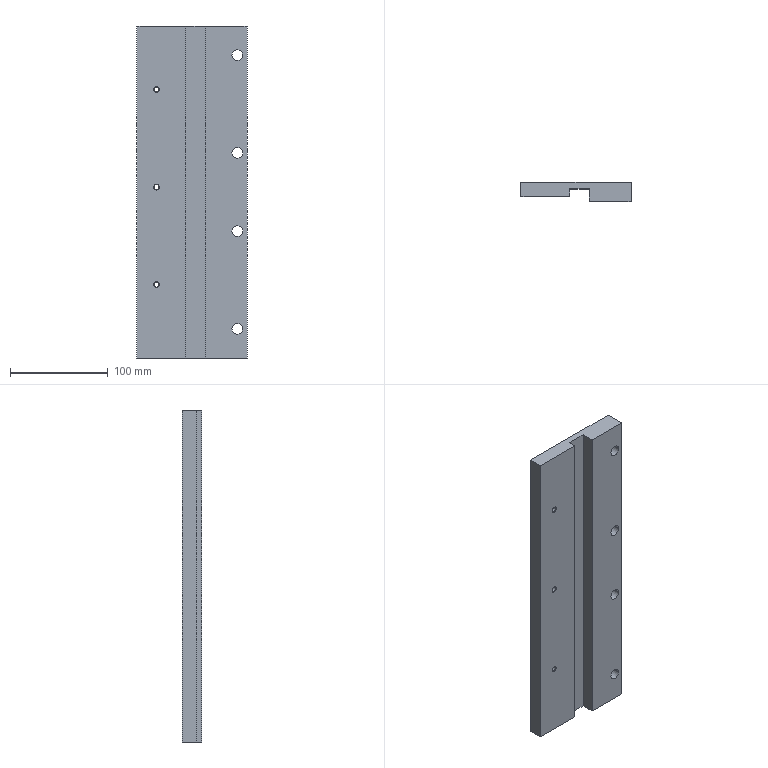Part | STEP file | 1 solid | 30 faces | box 112.747 x 19.5 x 340 mm | volume 565839 mm3 | cylinder 14 | plane 10 | cone 6 | commonest cylinder face diameters 11 x8 5 x6